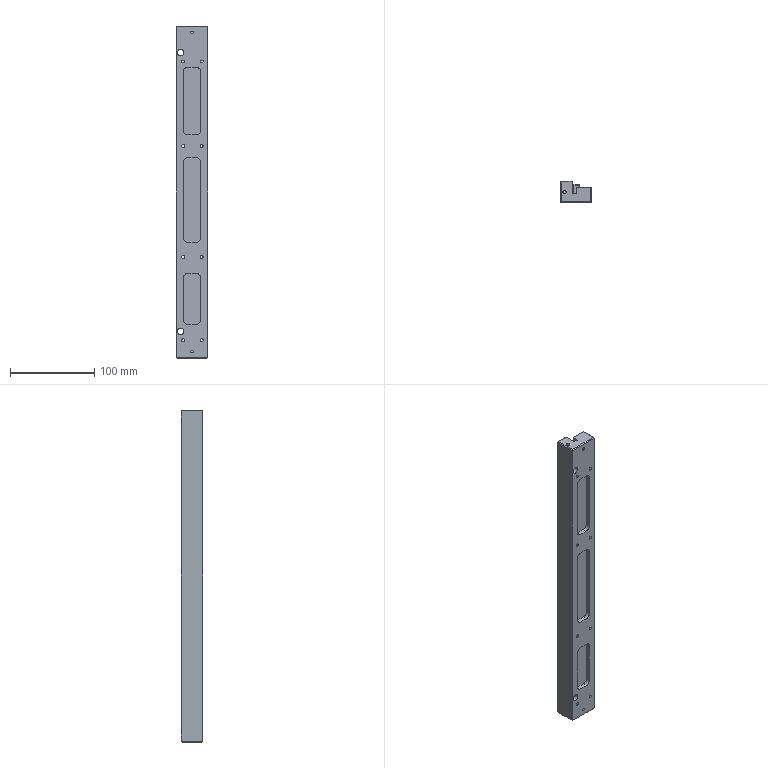Part | NX | features BREP 1 | 1 solid | 458 faces | box 37 x 25 x 393 mm | volume 229575 mm3 | plane 305 | cylinder 125 | cone 28 | commonest cylinder face diameters 4 x61 3.4 x16 6.7 x16 10 x13 2.5 x8 3 x4